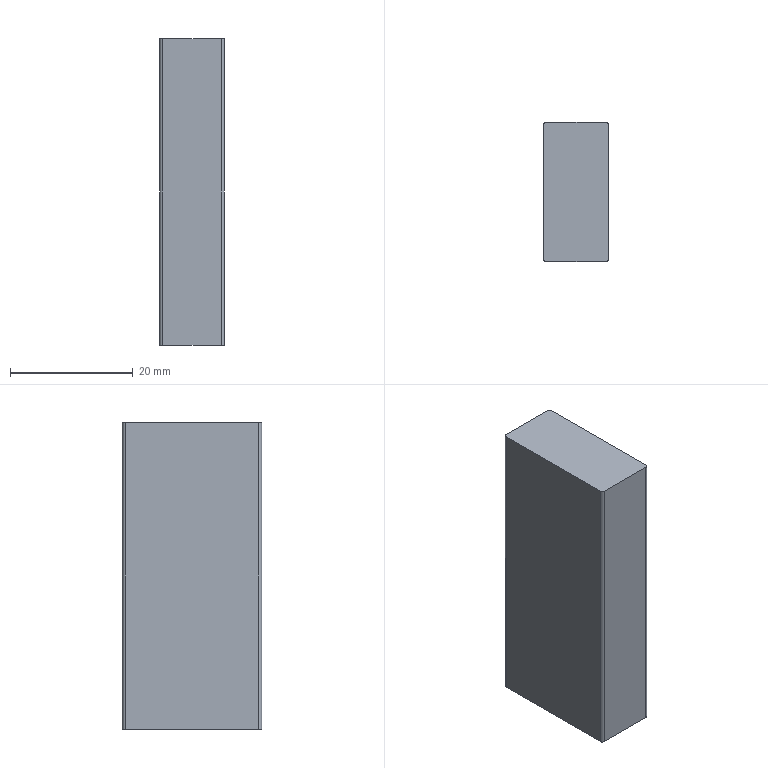Part | NX | features BREP 1 | 1 solid | 10 faces | box 10.558 x 22.702 x 50 mm | volume 11974 mm3 | plane 6 | cylinder 4 | commonest cylinder face diameters 1 x4
STEP:
#1=CARTESIAN_POINT('',(-4.779,11.351,-40.6));
#2=VERTEX_POINT('',#1);
#3=CARTESIAN_POINT('',(-5.279,10.851,-40.6));
#4=VERTEX_POINT('',#3);
#5=CARTESIAN_POINT('',(-4.779,10.851,-40.6));
#6=DIRECTION('',(0.,0.,1.));
#7=DIRECTION('',(1.,0.,0.));
#8=AXIS2_PLACEMENT_3D('',#5,#6,#7);
#9=CIRCLE('',#8,0.5);
#10=EDGE_CURVE('',#2,#4,#9,.T.);
#11=ORIENTED_EDGE('',*,*,#10,.F.);
#12=CARTESIAN_POINT('',(-4.779,11.351,-90.6));
#13=VERTEX_POINT('',#12);
#14=CARTESIAN_POINT('',(-4.779,11.351,-90.6));
#15=DIRECTION('',(0.,0.,1.));
#16=VECTOR('',#15,1000.);
#17=LINE('',#14,#16);
#18=EDGE_CURVE('',#13,#2,#17,.T.);
#19=ORIENTED_EDGE('',*,*,#18,.F.);
#20=CARTESIAN_POINT('',(-5.279,10.851,-90.6));
#21=VERTEX_POINT('',#20);
#22=CARTESIAN_POINT('',(-4.779,10.851,-90.6));
#23=DIRECTION('',(0.,0.,1.));
#24=DIRECTION('',(1.,0.,0.));
#25=AXIS2_PLACEMENT_3D('',#22,#23,#24);
#26=CIRCLE('',#25,0.5);
#27=EDGE_CURVE('',#13,#21,#26,.T.);
#28=ORIENTED_EDGE('',*,*,#27,.T.);
#29=CARTESIAN_POINT('',(-5.279,10.851,-90.6));
#30=DIRECTION('',(0.,0.,1.));
#31=VECTOR('',#30,1000.);
#32=LINE('',#29,#31);
#33=EDGE_CURVE('',#21,#4,#32,.T.);
#34=ORIENTED_EDGE('',*,*,#33,.T.);
#35=EDGE_LOOP('',(#11,#19,#28,#34));
#36=FACE_BOUND('',#35,.T.);
#37=CARTESIAN_POINT('',(-4.779,10.851,-90.6));
#38=DIRECTION('',(0.,0.,1.));
#39=DIRECTION('',(-1.,0.,0.));
#40=AXIS2_PLACEMENT_3D('',#37,#38,#39);
#41=CYLINDRICAL_SURFACE('',#40,0.5);
#42=ADVANCED_FACE('',(#36),#41,.T.);
#43=CARTESIAN_POINT('',(-5.279,-10.851,-40.6));
#44=VERTEX_POINT('',#43);
#45=CARTESIAN_POINT('',(-5.279,-10.851,-40.6));
#46=DIRECTION('',(0.,1.,0.));
#47=VECTOR('',#46,1000.);
#48=LINE('',#45,#47);
#49=EDGE_CURVE('',#44,#4,#48,.T.);
#50=ORIENTED_EDGE('',*,*,#49,.T.);
#51=ORIENTED_EDGE('',*,*,#33,.F.);
#52=CARTESIAN_POINT('',(-5.279,-10.851,-90.6));
#53=VERTEX_POINT('',#52);
#54=CARTESIAN_POINT('',(-5.279,-10.851,-90.6));
#55=DIRECTION('',(0.,1.,0.));
#56=VECTOR('',#55,1000.);
#57=LINE('',#54,#56);
#58=EDGE_CURVE('',#53,#21,#57,.T.);
#59=ORIENTED_EDGE('',*,*,#58,.F.);
#60=CARTESIAN_POINT('',(-5.279,-10.851,-90.6));
#61=DIRECTION('',(0.,0.,1.));
#62=VECTOR('',#61,1000.);
#63=LINE('',#60,#62);
#64=EDGE_CURVE('',#53,#44,#63,.T.);
#65=ORIENTED_EDGE('',*,*,#64,.T.);
#66=EDGE_LOOP('',(#50,#51,#59,#65));
#67=FACE_BOUND('',#66,.T.);
#68=CARTESIAN_POINT('',(-5.279,-10.851,-90.6));
#69=DIRECTION('',(1.,0.,0.));
#70=DIRECTION('',(0.,-1.,0.));
#71=AXIS2_PLACEMENT_3D('',#68,#69,#70);
#72=PLANE('',#71);
#73=ADVANCED_FACE('',(#67),#72,.F.);
#74=CARTESIAN_POINT('',(-4.779,-11.351,-40.6));
#75=VERTEX_POINT('',#74);
#76=CARTESIAN_POINT('',(-4.779,-10.851,-40.6));
#77=DIRECTION('',(0.,0.,1.));
#78=DIRECTION('',(1.,0.,0.));
#79=AXIS2_PLACEMENT_3D('',#76,#77,#78);
#80=CIRCLE('',#79,0.5);
#81=EDGE_CURVE('',#44,#75,#80,.T.);
#82=ORIENTED_EDGE('',*,*,#81,.F.);
#83=ORIENTED_EDGE('',*,*,#64,.F.);
#84=CARTESIAN_POINT('',(-4.779,-11.351,-90.6));
#85=VERTEX_POINT('',#84);
#86=CARTESIAN_POINT('',(-4.779,-10.851,-90.6));
#87=DIRECTION('',(0.,0.,1.));
#88=DIRECTION('',(1.,0.,0.));
#89=AXIS2_PLACEMENT_3D('',#86,#87,#88);
#90=CIRCLE('',#89,0.5);
#91=EDGE_CURVE('',#53,#85,#90,.T.);
#92=ORIENTED_EDGE('',*,*,#91,.T.);
#93=CARTESIAN_POINT('',(-4.779,-11.351,-90.6));
#94=DIRECTION('',(0.,0.,1.));
#95=VECTOR('',#94,1000.);
#96=LINE('',#93,#95);
#97=EDGE_CURVE('',#85,#75,#96,.T.);
#98=ORIENTED_EDGE('',*,*,#97,.T.);
#99=EDGE_LOOP('',(#82,#83,#92,#98));
#100=FACE_BOUND('',#99,.T.);
#101=CARTESIAN_POINT('',(-4.779,-10.851,-90.6));
#102=DIRECTION('',(0.,0.,1.));
#103=DIRECTION('',(-1.,0.,0.));
#104=AXIS2_PLACEMENT_3D('',#101,#102,#103);
#105=CYLINDRICAL_SURFACE('',#104,0.5);
#106=ADVANCED_FACE('',(#100),#105,.T.);
#107=CARTESIAN_POINT('',(4.779,-11.351,-40.6));
#108=VERTEX_POINT('',#107);
#109=CARTESIAN_POINT('',(4.779,-11.351,-40.6));
#110=DIRECTION('',(-1.,0.,0.));
#111=VECTOR('',#110,1000.);
#112=LINE('',#109,#111);
#113=EDGE_CURVE('',#108,#75,#112,.T.);
#114=ORIENTED_EDGE('',*,*,#113,.T.);
#115=ORIENTED_EDGE('',*,*,#97,.F.);
#116=CARTESIAN_POINT('',(4.779,-11.351,-90.6));
#117=VERTEX_POINT('',#116);
#118=CARTESIAN_POINT('',(4.779,-11.351,-90.6));
#119=DIRECTION('',(-1.,0.,0.));
#120=VECTOR('',#119,1000.);
#121=LINE('',#118,#120);
#122=EDGE_CURVE('',#117,#85,#121,.T.);
#123=ORIENTED_EDGE('',*,*,#122,.F.);
#124=CARTESIAN_POINT('',(4.779,-11.351,-90.6));
#125=DIRECTION('',(0.,0.,1.));
#126=VECTOR('',#125,1000.);
#127=LINE('',#124,#126);
#128=EDGE_CURVE('',#117,#108,#127,.T.);
#129=ORIENTED_EDGE('',*,*,#128,.T.);
#130=EDGE_LOOP('',(#114,#115,#123,#129));
#131=FACE_BOUND('',#130,.T.);
#132=CARTESIAN_POINT('',(4.779,-11.351,-90.6));
#133=DIRECTION('',(0.,1.,0.));
#134=DIRECTION('',(1.,0.,0.));
#135=AXIS2_PLACEMENT_3D('',#132,#133,#134);
#136=PLANE('',#135);
#137=ADVANCED_FACE('',(#131),#136,.F.);
#138=CARTESIAN_POINT('',(5.279,-10.851,-40.6));
#139=VERTEX_POINT('',#138);
#140=CARTESIAN_POINT('',(4.779,-10.851,-40.6));
#141=DIRECTION('',(0.,0.,1.));
#142=DIRECTION('',(1.,0.,0.));
#143=AXIS2_PLACEMENT_3D('',#140,#141,#142);
#144=CIRCLE('',#143,0.5);
#145=EDGE_CURVE('',#108,#139,#144,.T.);
#146=ORIENTED_EDGE('',*,*,#145,.F.);
#147=ORIENTED_EDGE('',*,*,#128,.F.);
#148=CARTESIAN_POINT('',(5.279,-10.851,-90.6));
#149=VERTEX_POINT('',#148);
#150=CARTESIAN_POINT('',(4.779,-10.851,-90.6));
#151=DIRECTION('',(0.,0.,1.));
#152=DIRECTION('',(1.,0.,0.));
#153=AXIS2_PLACEMENT_3D('',#150,#151,#152);
#154=CIRCLE('',#153,0.5);
#155=EDGE_CURVE('',#117,#149,#154,.T.);
#156=ORIENTED_EDGE('',*,*,#155,.T.);
#157=CARTESIAN_POINT('',(5.279,-10.851,-90.6));
#158=DIRECTION('',(0.,0.,1.));
#159=VECTOR('',#158,1000.);
#160=LINE('',#157,#159);
#161=EDGE_CURVE('',#149,#139,#160,.T.);
#162=ORIENTED_EDGE('',*,*,#161,.T.);
#163=EDGE_LOOP('',(#146,#147,#156,#162));
#164=FACE_BOUND('',#163,.T.);
#165=CARTESIAN_POINT('',(4.779,-10.851,-90.6));
#166=DIRECTION('',(0.,0.,1.));
#167=DIRECTION('',(-1.,0.,0.));
#168=AXIS2_PLACEMENT_3D('',#165,#166,#167);
#169=CYLINDRICAL_SURFACE('',#168,0.5);
#170=ADVANCED_FACE('',(#164),#169,.T.);
#171=CARTESIAN_POINT('',(5.279,10.851,-40.6));
#172=VERTEX_POINT('',#171);
#173=CARTESIAN_POINT('',(5.279,10.851,-40.6));
#174=DIRECTION('',(0.,-1.,0.));
#175=VECTOR('',#174,1000.);
#176=LINE('',#173,#175);
#177=EDGE_CURVE('',#172,#139,#176,.T.);
#178=ORIENTED_EDGE('',*,*,#177,.T.);
#179=ORIENTED_EDGE('',*,*,#161,.F.);
#180=CARTESIAN_POINT('',(5.279,10.851,-90.6));
#181=VERTEX_POINT('',#180);
#182=CARTESIAN_POINT('',(5.279,10.851,-90.6));
#183=DIRECTION('',(0.,-1.,0.));
#184=VECTOR('',#183,1000.);
#185=LINE('',#182,#184);
#186=EDGE_CURVE('',#181,#149,#185,.T.);
#187=ORIENTED_EDGE('',*,*,#186,.F.);
#188=CARTESIAN_POINT('',(5.279,10.851,-90.6));
#189=DIRECTION('',(0.,0.,1.));
#190=VECTOR('',#189,1000.);
#191=LINE('',#188,#190);
#192=EDGE_CURVE('',#181,#172,#191,.T.);
#193=ORIENTED_EDGE('',*,*,#192,.T.);
#194=EDGE_LOOP('',(#178,#179,#187,#193));
#195=FACE_BOUND('',#194,.T.);
#196=CARTESIAN_POINT('',(5.279,10.851,-90.6));
#197=DIRECTION('',(-1.,0.,0.));
#198=DIRECTION('',(0.,0.,-1.));
#199=AXIS2_PLACEMENT_3D('',#196,#197,#198);
#200=PLANE('',#199);
#201=ADVANCED_FACE('',(#195),#200,.F.);
#202=CARTESIAN_POINT('',(4.779,11.351,-40.6));
#203=VERTEX_POINT('',#202);
#204=CARTESIAN_POINT('',(4.779,10.851,-40.6));
#205=DIRECTION('',(0.,0.,1.));
#206=DIRECTION('',(1.,0.,0.));
#207=AXIS2_PLACEMENT_3D('',#204,#205,#206);
#208=CIRCLE('',#207,0.5);
#209=EDGE_CURVE('',#172,#203,#208,.T.);
#210=ORIENTED_EDGE('',*,*,#209,.F.);
#211=ORIENTED_EDGE('',*,*,#192,.F.);
#212=CARTESIAN_POINT('',(4.779,11.351,-90.6));
#213=VERTEX_POINT('',#212);
#214=CARTESIAN_POINT('',(4.779,10.851,-90.6));
#215=DIRECTION('',(0.,0.,1.));
#216=DIRECTION('',(1.,0.,0.));
#217=AXIS2_PLACEMENT_3D('',#214,#215,#216);
#218=CIRCLE('',#217,0.5);
#219=EDGE_CURVE('',#181,#213,#218,.T.);
#220=ORIENTED_EDGE('',*,*,#219,.T.);
#221=CARTESIAN_POINT('',(4.779,11.351,-90.6));
#222=DIRECTION('',(0.,0.,1.));
#223=VECTOR('',#222,1000.);
#224=LINE('',#221,#223);
#225=EDGE_CURVE('',#213,#203,#224,.T.);
#226=ORIENTED_EDGE('',*,*,#225,.T.);
#227=EDGE_LOOP('',(#210,#211,#220,#226));
#228=FACE_BOUND('',#227,.T.);
#229=CARTESIAN_POINT('',(4.779,10.851,-90.6));
#230=DIRECTION('',(0.,0.,1.));
#231=DIRECTION('',(-1.,0.,0.));
#232=AXIS2_PLACEMENT_3D('',#229,#230,#231);
#233=CYLINDRICAL_SURFACE('',#232,0.5);
#234=ADVANCED_FACE('',(#228),#233,.T.);
#235=CARTESIAN_POINT('',(-4.779,11.351,-40.6));
#236=DIRECTION('',(1.,0.,0.));
#237=VECTOR('',#236,1000.);
#238=LINE('',#235,#237);
#239=EDGE_CURVE('',#2,#203,#238,.T.);
#240=ORIENTED_EDGE('',*,*,#239,.T.);
#241=ORIENTED_EDGE('',*,*,#225,.F.);
#242=CARTESIAN_POINT('',(-4.779,11.351,-90.6));
#243=DIRECTION('',(1.,0.,0.));
#244=VECTOR('',#243,1000.);
#245=LINE('',#242,#244);
#246=EDGE_CURVE('',#13,#213,#245,.T.);
#247=ORIENTED_EDGE('',*,*,#246,.F.);
#248=ORIENTED_EDGE('',*,*,#18,.T.);
#249=EDGE_LOOP('',(#240,#241,#247,#248));
#250=FACE_BOUND('',#249,.T.);
#251=CARTESIAN_POINT('',(-4.779,11.351,-90.6));
#252=DIRECTION('',(0.,-1.,0.));
#253=DIRECTION('',(-1.,0.,0.));
#254=AXIS2_PLACEMENT_3D('',#251,#252,#253);
#255=PLANE('',#254);
#256=ADVANCED_FACE('',(#250),#255,.F.);
#257=ORIENTED_EDGE('',*,*,#27,.F.);
#258=ORIENTED_EDGE('',*,*,#246,.T.);
#259=ORIENTED_EDGE('',*,*,#219,.F.);
#260=ORIENTED_EDGE('',*,*,#186,.T.);
#261=ORIENTED_EDGE('',*,*,#155,.F.);
#262=ORIENTED_EDGE('',*,*,#122,.T.);
#263=ORIENTED_EDGE('',*,*,#91,.F.);
#264=ORIENTED_EDGE('',*,*,#58,.T.);
#265=EDGE_LOOP('',(#257,#258,#259,#260,#261,#262,#263,#264));
#266=FACE_BOUND('',#265,.T.);
#267=CARTESIAN_POINT('',(-4.779,10.851,-90.6));
#268=DIRECTION('',(0.,0.,1.));
#269=DIRECTION('',(-1.,0.,0.));
#270=AXIS2_PLACEMENT_3D('',#267,#268,#269);
#271=PLANE('',#270);
#272=ADVANCED_FACE('',(#266),#271,.F.);
#273=ORIENTED_EDGE('',*,*,#10,.T.);
#274=ORIENTED_EDGE('',*,*,#49,.F.);
#275=ORIENTED_EDGE('',*,*,#81,.T.);
#276=ORIENTED_EDGE('',*,*,#113,.F.);
#277=ORIENTED_EDGE('',*,*,#145,.T.);
#278=ORIENTED_EDGE('',*,*,#177,.F.);
#279=ORIENTED_EDGE('',*,*,#209,.T.);
#280=ORIENTED_EDGE('',*,*,#239,.F.);
#281=EDGE_LOOP('',(#273,#274,#275,#276,#277,#278,#279,#280));
#282=FACE_BOUND('',#281,.T.);
#283=CARTESIAN_POINT('',(-4.779,10.851,-40.6));
#284=DIRECTION('',(0.,0.,1.));
#285=DIRECTION('',(-1.,0.,0.));
#286=AXIS2_PLACEMENT_3D('',#283,#284,#285);
#287=PLANE('',#286);
#288=ADVANCED_FACE('',(#282),#287,.T.);
#289=CLOSED_SHELL('',(#42,#73,#106,#137,#170,#201,#234,#256,#272,#288));
#290=MANIFOLD_SOLID_BREP('',#289);
#291=(LENGTH_UNIT()NAMED_UNIT(*)SI_UNIT(.MILLI.,.METRE.));
#292=UNCERTAINTY_MEASURE_WITH_UNIT(LENGTH_MEASURE(0.00001),#291,'','');
#293=(NAMED_UNIT(*)PLANE_ANGLE_UNIT()SI_UNIT($,.RADIAN.));
#294=(NAMED_UNIT(*)SI_UNIT($,.STERADIAN.)SOLID_ANGLE_UNIT());
#295=(GEOMETRIC_REPRESENTATION_CONTEXT(3)GLOBAL_UNCERTAINTY_ASSIGNED_CONTEXT((#292))GLOBAL_UNIT_ASSIGNED_CONTEXT((#291,#293,#294))REPRESENTATION_CONTEXT('',''));
#296=ADVANCED_BREP_SHAPE_REPRESENTATION('',(#290),#295);